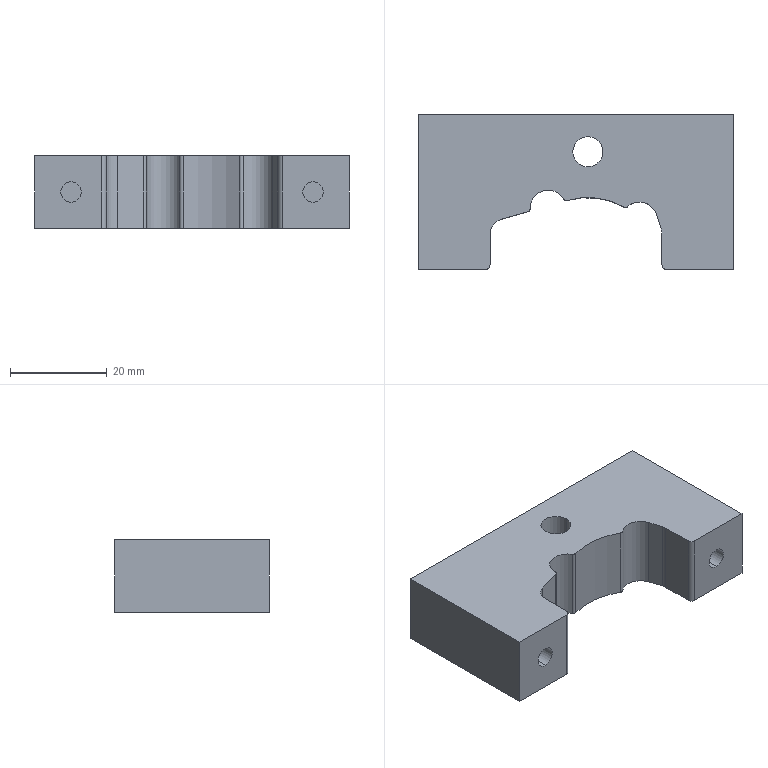CAM job | Mastercam | 3-axis milling, drilling
Tools:
tool_number,name,type,diameter_mm,corner_radius_mm,flutes,flute_length_mm,overall_length_mm,shoulder_length_mm,holder_diameter_mm,length_offset,diameter_offset,default_rpm,default_feed_mm_min,default_plunge_mm_min,coolant
1,50 Facing,end mill,50,0,4,5,50,18,50,1,1,5000,700,2000,COOL_OFF
2,16 Roughing cutter,end mill,16,0,4,25,50,25,50,2,2,5500,2000,2000,COOL_OFF
3,5 Flat End Mill Finish,end mill,5,0,4,21,21,21,50,3,3,2000,240,600,COOL_OFF
4,16 Finish cutter,end mill,16,0,4,25,50,25,50,4,4,4000,800,2000,COOL_OFF
5,8 Chamfer Mill,chamfer mill,8,0,4,25,30,30,50,5,5,3125,375,600,COOL_OFF
6,5 Drill,drill,5,0,2,25,50,40,50,6,6,1200,144,600,COOL_OFF
7,M6 x 1 RH Tap,drill,6,0,2,24,62,24,50,7,7,1000,1000,600,COOL_OFF
8,8.5 Drill,drill,8.5,0,2,25,50,40,50,8,8,706,84.72,600,COOL_OFF
9,8 Flat End Mill Rough,end mill,8,0,4,25,25,25,50,9,9,1250,150,600,COOL_OFF
10,8 Flat End Mill Finish,end mill,8,0,4,25,25,25,50,10,10,1250,150,600,COOL_OFF
11,6.2 Drill,drill,6.2,0,2,25,50,40,50,11,11,968,116.16,600,COOL_OFF
11,7 Drill,drill,7,0,2,25,50,40,50,11,11,857,102.84,600,COOL_OFF
12,12 Plunge cutter,end mill,12,0,4,25,25,25,50,12,12,833,99.96,600,COOL_OFF
13,6.8 Drill,drill,6.8,0,2,25,50,40,50,13,13,882,105.84,600,COOL_OFF
14,M8 x 1.25 RH Tap,drill,8,0,2,30,70,30,50,14,14,750,937.5,600,COOL_OFF
15,4.2 Drill,drill,4.2,0,2,25,50,40,50,15,15,1429,171.48,600,COOL_OFF
16,M5 x 0.8 RH Tap,drill,5,0,2,22,60,22,50,16,16,1200,960.0,600,COOL_OFF
Operations:
seq,operation,operation_type,tool_number,tool_name,tool_diameter_mm,spindle_rpm,feed_mm_min,plunge_mm_min,retract_mm_min,cycle_time_s,wcs,posted,nc_file
1,Facing - [WCS: Top] - [Tplane: Top],Facing,1,50 Facing,50,5000,700,2000,5000,13.388,Top,yes,.nc
2,2D High Speed (2D Dynamic Mill) - [WCS: Top] - [Tplane: Top],HighSpeed2D,9,8 Flat End Mill Rough,8,6000,4000,2000,5000,80.802,Top,yes,.nc
3,2D High Speed (2D Dynamic Rest Mill) - [WCS: Top] - [Tplane: Top],HighSpeed2D,3,5 Flat End Mill Finish,5,5500,1500,2000,1200,15.277,Top,yes,.nc
4,Drill/Counterbore - [WCS: Top] - [Tplane: Top],Drill,5,8 Chamfer Mill,8,3000,300,600,1200,1.31,Top,yes,.nc
5,Peck Drill - [WCS: Top] - [Tplane: Top],Drill,11,7 Drill,7,3000,300,600,1200,5.347,Top,yes,.nc
6,Contour (2D chamfer) - [WCS: Top] - [Tplane: Top],Contour,5,8 Chamfer Mill,8,5000,1000,2000,1200,14.359,Top,yes,.nc
7,Contour (2D) - [WCS: Top] - [Tplane: Top],Contour,10,8 Flat End Mill Finish,8,5000,600,2000,1200,51.004,Top,yes,.nc
8,Contour (2D) - [WCS: Top] - [Tplane: Top],Contour,3,5 Flat End Mill Finish,5,5000,600,2000,1200,13.293,Top,yes,.nc
9,Facing - [WCS: Top] - [Tplane: Plane],Facing,1,50 Facing,50,5000,1500,2000,5000,30.653,Top,yes,.nc
10,Facing - [WCS: Top] - [Tplane: Plane],Facing,1,50 Facing,50,5000,700,2000,5000,13.388,Top,yes,.nc
11,Drill/Counterbore - [WCS: Top] - [Tplane: Plane],Drill,5,8 Chamfer Mill,8,3000,400,600,1200,1.105,Top,yes,.nc
12,Contour (2D chamfer) - [WCS: Top] - [Tplane: Plane],Contour,5,8 Chamfer Mill,8,5000,1000,2000,1200,14.362,Top,yes,.nc
13,Drill/Counterbore - [WCS: Top] - [Tplane: Plane-1],Drill,5,8 Chamfer Mill,8,3000,300,600,1200,2.17,Top,yes,.nc
14,Peck Drill - [WCS: Top] - [Tplane: Plane-1],Drill,15,4.2 Drill,4.2,3000,300,600,1200,9.286,Top,yes,.nc
15,Tap - [WCS: Top] - [Tplane: Plane-1],Drill,16,M5 x 0.8 RH Tap,5,400,320.0,600,1200,28.595,Top,yes,.nc